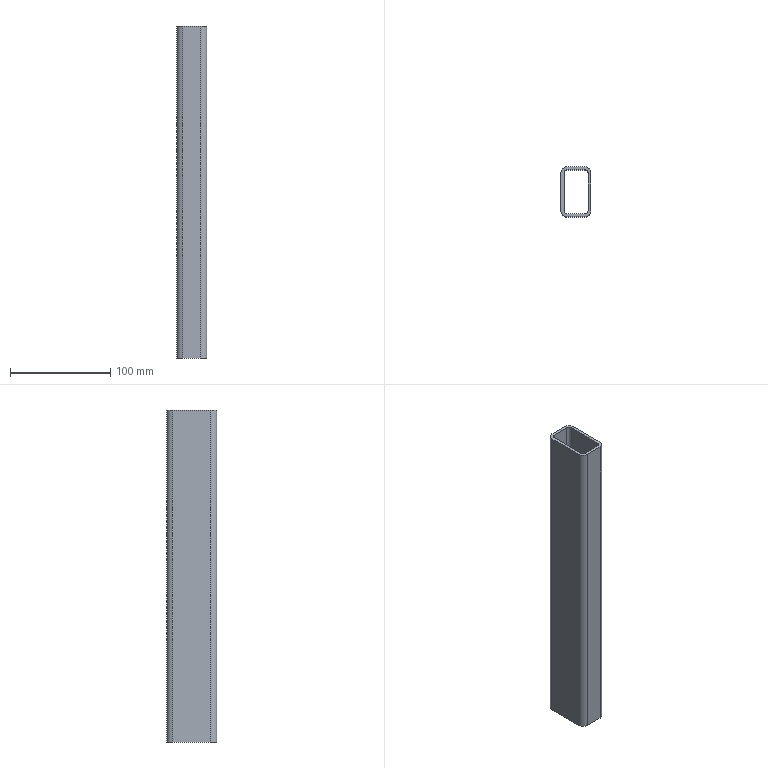Part | STEP file | ISO 10799-2 50x30x3 1784900903573 | 1 solid | 18 faces | box 30 x 50 x 332 mm | volume 139713 mm3 | plane 10 | cylinder 8 | commonest cylinder face diameters 6 x4 12 x4
STEP:
#1=CARTESIAN_POINT('',(-9.,-22.,372.));
#2=VERTEX_POINT('',#1);
#3=CARTESIAN_POINT('',(9.,-22.,372.));
#4=VERTEX_POINT('',#3);
#5=CARTESIAN_POINT('',(4.5,-22.,372.));
#6=DIRECTION('',(1.,0.,0.));
#7=VECTOR('',#6,10.);
#8=LINE('',#5,#7);
#9=EDGE_CURVE('',#2,#4,#8,.T.);
#10=ORIENTED_EDGE('',*,*,#9,.T.);
#11=CARTESIAN_POINT('',(9.,-22.,40.));
#12=VERTEX_POINT('',#11);
#13=CARTESIAN_POINT('',(9.,-22.,0.));
#14=DIRECTION('',(0.,0.,1.));
#15=VECTOR('',#14,10.);
#16=LINE('',#13,#15);
#17=EDGE_CURVE('',#12,#4,#16,.T.);
#18=ORIENTED_EDGE('',*,*,#17,.F.);
#19=CARTESIAN_POINT('',(-9.,-22.,40.));
#20=VERTEX_POINT('',#19);
#21=CARTESIAN_POINT('',(4.5,-22.,40.));
#22=DIRECTION('',(1.,0.,0.));
#23=VECTOR('',#22,10.);
#24=LINE('',#21,#23);
#25=EDGE_CURVE('',#20,#12,#24,.T.);
#26=ORIENTED_EDGE('',*,*,#25,.F.);
#27=CARTESIAN_POINT('',(-9.,-22.,0.));
#28=DIRECTION('',(0.,0.,1.));
#29=VECTOR('',#28,10.);
#30=LINE('',#27,#29);
#31=EDGE_CURVE('',#20,#2,#30,.T.);
#32=ORIENTED_EDGE('',*,*,#31,.T.);
#33=EDGE_LOOP('',(#10,#18,#26,#32));
#34=FACE_OUTER_BOUND('',#33,.T.);
#35=CARTESIAN_POINT('',(9.,-22.,0.));
#36=DIRECTION('',(0.,-1.,0.));
#37=DIRECTION('',(0.,0.,-1.));
#38=AXIS2_PLACEMENT_3D('',#35,#36,#37);
#39=PLANE('',#38);
#40=ADVANCED_FACE('',(#34),#39,.F.);
#41=CARTESIAN_POINT('',(12.,-19.,372.));
#42=VERTEX_POINT('',#41);
#43=CARTESIAN_POINT('',(9.,-19.,372.));
#44=DIRECTION('',(0.,0.,1.));
#45=DIRECTION('',(0.,1.,0.));
#46=AXIS2_PLACEMENT_3D('',#43,#44,#45);
#47=CIRCLE('',#46,3.);
#48=EDGE_CURVE('',#4,#42,#47,.T.);
#49=ORIENTED_EDGE('',*,*,#48,.T.);
#50=CARTESIAN_POINT('',(12.,-19.,40.));
#51=VERTEX_POINT('',#50);
#52=CARTESIAN_POINT('',(12.,-19.,0.));
#53=DIRECTION('',(0.,0.,1.));
#54=VECTOR('',#53,10.);
#55=LINE('',#52,#54);
#56=EDGE_CURVE('',#51,#42,#55,.T.);
#57=ORIENTED_EDGE('',*,*,#56,.F.);
#58=CARTESIAN_POINT('',(9.,-19.,40.));
#59=DIRECTION('',(0.,0.,1.));
#60=DIRECTION('',(0.,1.,0.));
#61=AXIS2_PLACEMENT_3D('',#58,#59,#60);
#62=CIRCLE('',#61,3.);
#63=EDGE_CURVE('',#12,#51,#62,.T.);
#64=ORIENTED_EDGE('',*,*,#63,.F.);
#65=ORIENTED_EDGE('',*,*,#17,.T.);
#66=EDGE_LOOP('',(#49,#57,#64,#65));
#67=FACE_OUTER_BOUND('',#66,.T.);
#68=CARTESIAN_POINT('',(9.,-19.,0.));
#69=DIRECTION('',(0.,0.,1.));
#70=DIRECTION('',(0.,1.,0.));
#71=AXIS2_PLACEMENT_3D('',#68,#69,#70);
#72=CYLINDRICAL_SURFACE('',#71,3.);
#73=ADVANCED_FACE('',(#67),#72,.F.);
#74=CARTESIAN_POINT('',(12.,19.,372.));
#75=VERTEX_POINT('',#74);
#76=CARTESIAN_POINT('',(12.,9.5,372.));
#77=DIRECTION('',(0.,1.,0.));
#78=VECTOR('',#77,10.);
#79=LINE('',#76,#78);
#80=EDGE_CURVE('',#42,#75,#79,.T.);
#81=ORIENTED_EDGE('',*,*,#80,.T.);
#82=CARTESIAN_POINT('',(12.,19.,40.));
#83=VERTEX_POINT('',#82);
#84=CARTESIAN_POINT('',(12.,19.,0.));
#85=DIRECTION('',(0.,0.,1.));
#86=VECTOR('',#85,10.);
#87=LINE('',#84,#86);
#88=EDGE_CURVE('',#83,#75,#87,.T.);
#89=ORIENTED_EDGE('',*,*,#88,.F.);
#90=CARTESIAN_POINT('',(12.,9.5,40.));
#91=DIRECTION('',(0.,1.,0.));
#92=VECTOR('',#91,10.);
#93=LINE('',#90,#92);
#94=EDGE_CURVE('',#51,#83,#93,.T.);
#95=ORIENTED_EDGE('',*,*,#94,.F.);
#96=ORIENTED_EDGE('',*,*,#56,.T.);
#97=EDGE_LOOP('',(#81,#89,#95,#96));
#98=FACE_OUTER_BOUND('',#97,.T.);
#99=CARTESIAN_POINT('',(12.,19.,0.));
#100=DIRECTION('',(1.,0.,0.));
#101=DIRECTION('',(0.,0.,-1.));
#102=AXIS2_PLACEMENT_3D('',#99,#100,#101);
#103=PLANE('',#102);
#104=ADVANCED_FACE('',(#98),#103,.F.);
#105=CARTESIAN_POINT('',(9.,22.,372.));
#106=VERTEX_POINT('',#105);
#107=CARTESIAN_POINT('',(9.,19.,372.));
#108=DIRECTION('',(0.,0.,1.));
#109=DIRECTION('',(-1.,0.,0.));
#110=AXIS2_PLACEMENT_3D('',#107,#108,#109);
#111=CIRCLE('',#110,3.);
#112=EDGE_CURVE('',#75,#106,#111,.T.);
#113=ORIENTED_EDGE('',*,*,#112,.T.);
#114=CARTESIAN_POINT('',(9.,22.,40.));
#115=VERTEX_POINT('',#114);
#116=CARTESIAN_POINT('',(9.,22.,0.));
#117=DIRECTION('',(0.,0.,1.));
#118=VECTOR('',#117,10.);
#119=LINE('',#116,#118);
#120=EDGE_CURVE('',#115,#106,#119,.T.);
#121=ORIENTED_EDGE('',*,*,#120,.F.);
#122=CARTESIAN_POINT('',(9.,19.,40.));
#123=DIRECTION('',(0.,0.,1.));
#124=DIRECTION('',(-1.,0.,0.));
#125=AXIS2_PLACEMENT_3D('',#122,#123,#124);
#126=CIRCLE('',#125,3.);
#127=EDGE_CURVE('',#83,#115,#126,.T.);
#128=ORIENTED_EDGE('',*,*,#127,.F.);
#129=ORIENTED_EDGE('',*,*,#88,.T.);
#130=EDGE_LOOP('',(#113,#121,#128,#129));
#131=FACE_OUTER_BOUND('',#130,.T.);
#132=CARTESIAN_POINT('',(9.,19.,0.));
#133=DIRECTION('',(0.,0.,1.));
#134=DIRECTION('',(-1.,0.,0.));
#135=AXIS2_PLACEMENT_3D('',#132,#133,#134);
#136=CYLINDRICAL_SURFACE('',#135,3.);
#137=ADVANCED_FACE('',(#131),#136,.F.);
#138=CARTESIAN_POINT('',(15.,19.,372.));
#139=VERTEX_POINT('',#138);
#140=CARTESIAN_POINT('',(15.,-19.,372.));
#141=VERTEX_POINT('',#140);
#142=CARTESIAN_POINT('',(15.,9.5,372.));
#143=DIRECTION('',(0.,-1.,0.));
#144=VECTOR('',#143,10.);
#145=LINE('',#142,#144);
#146=EDGE_CURVE('',#139,#141,#145,.T.);
#147=ORIENTED_EDGE('',*,*,#146,.T.);
#148=CARTESIAN_POINT('',(15.,-19.,40.));
#149=VERTEX_POINT('',#148);
#150=CARTESIAN_POINT('',(15.,-19.,0.));
#151=DIRECTION('',(0.,0.,1.));
#152=VECTOR('',#151,10.);
#153=LINE('',#150,#152);
#154=EDGE_CURVE('',#149,#141,#153,.T.);
#155=ORIENTED_EDGE('',*,*,#154,.F.);
#156=CARTESIAN_POINT('',(15.,19.,40.));
#157=VERTEX_POINT('',#156);
#158=CARTESIAN_POINT('',(15.,9.5,40.));
#159=DIRECTION('',(0.,-1.,0.));
#160=VECTOR('',#159,10.);
#161=LINE('',#158,#160);
#162=EDGE_CURVE('',#157,#149,#161,.T.);
#163=ORIENTED_EDGE('',*,*,#162,.F.);
#164=CARTESIAN_POINT('',(15.,19.,0.));
#165=DIRECTION('',(0.,0.,1.));
#166=VECTOR('',#165,10.);
#167=LINE('',#164,#166);
#168=EDGE_CURVE('',#157,#139,#167,.T.);
#169=ORIENTED_EDGE('',*,*,#168,.T.);
#170=EDGE_LOOP('',(#147,#155,#163,#169));
#171=FACE_OUTER_BOUND('',#170,.T.);
#172=CARTESIAN_POINT('',(15.,19.,0.));
#173=DIRECTION('',(1.,0.,0.));
#174=DIRECTION('',(0.,0.,-1.));
#175=AXIS2_PLACEMENT_3D('',#172,#173,#174);
#176=PLANE('',#175);
#177=ADVANCED_FACE('',(#171),#176,.T.);
#178=CARTESIAN_POINT('',(9.,-25.,372.));
#179=VERTEX_POINT('',#178);
#180=CARTESIAN_POINT('',(9.,-19.,372.));
#181=DIRECTION('',(0.,0.,-1.));
#182=DIRECTION('',(0.,1.,0.));
#183=AXIS2_PLACEMENT_3D('',#180,#181,#182);
#184=CIRCLE('',#183,6.);
#185=EDGE_CURVE('',#141,#179,#184,.T.);
#186=ORIENTED_EDGE('',*,*,#185,.T.);
#187=CARTESIAN_POINT('',(9.,-25.,40.));
#188=VERTEX_POINT('',#187);
#189=CARTESIAN_POINT('',(9.,-25.,0.));
#190=DIRECTION('',(0.,0.,1.));
#191=VECTOR('',#190,10.);
#192=LINE('',#189,#191);
#193=EDGE_CURVE('',#188,#179,#192,.T.);
#194=ORIENTED_EDGE('',*,*,#193,.F.);
#195=CARTESIAN_POINT('',(9.,-19.,40.));
#196=DIRECTION('',(0.,0.,-1.));
#197=DIRECTION('',(0.,1.,0.));
#198=AXIS2_PLACEMENT_3D('',#195,#196,#197);
#199=CIRCLE('',#198,6.);
#200=EDGE_CURVE('',#149,#188,#199,.T.);
#201=ORIENTED_EDGE('',*,*,#200,.F.);
#202=ORIENTED_EDGE('',*,*,#154,.T.);
#203=EDGE_LOOP('',(#186,#194,#201,#202));
#204=FACE_OUTER_BOUND('',#203,.T.);
#205=CARTESIAN_POINT('',(9.,-19.,0.));
#206=DIRECTION('',(0.,0.,1.));
#207=DIRECTION('',(0.,1.,0.));
#208=AXIS2_PLACEMENT_3D('',#205,#206,#207);
#209=CYLINDRICAL_SURFACE('',#208,6.);
#210=ADVANCED_FACE('',(#204),#209,.T.);
#211=CARTESIAN_POINT('',(-9.,-25.,372.));
#212=VERTEX_POINT('',#211);
#213=CARTESIAN_POINT('',(4.5,-25.,372.));
#214=DIRECTION('',(-1.,0.,0.));
#215=VECTOR('',#214,10.);
#216=LINE('',#213,#215);
#217=EDGE_CURVE('',#179,#212,#216,.T.);
#218=ORIENTED_EDGE('',*,*,#217,.T.);
#219=CARTESIAN_POINT('',(-9.,-25.,40.));
#220=VERTEX_POINT('',#219);
#221=CARTESIAN_POINT('',(-9.,-25.,0.));
#222=DIRECTION('',(0.,0.,1.));
#223=VECTOR('',#222,10.);
#224=LINE('',#221,#223);
#225=EDGE_CURVE('',#220,#212,#224,.T.);
#226=ORIENTED_EDGE('',*,*,#225,.F.);
#227=CARTESIAN_POINT('',(4.5,-25.,40.));
#228=DIRECTION('',(-1.,0.,0.));
#229=VECTOR('',#228,10.);
#230=LINE('',#227,#229);
#231=EDGE_CURVE('',#188,#220,#230,.T.);
#232=ORIENTED_EDGE('',*,*,#231,.F.);
#233=ORIENTED_EDGE('',*,*,#193,.T.);
#234=EDGE_LOOP('',(#218,#226,#232,#233));
#235=FACE_OUTER_BOUND('',#234,.T.);
#236=CARTESIAN_POINT('',(9.,-25.,0.));
#237=DIRECTION('',(0.,-1.,0.));
#238=DIRECTION('',(0.,0.,-1.));
#239=AXIS2_PLACEMENT_3D('',#236,#237,#238);
#240=PLANE('',#239);
#241=ADVANCED_FACE('',(#235),#240,.T.);
#242=CARTESIAN_POINT('',(-15.,-19.,372.));
#243=VERTEX_POINT('',#242);
#244=CARTESIAN_POINT('',(-9.,-19.,372.));
#245=DIRECTION('',(0.,0.,-1.));
#246=DIRECTION('',(1.,0.,0.));
#247=AXIS2_PLACEMENT_3D('',#244,#245,#246);
#248=CIRCLE('',#247,6.);
#249=EDGE_CURVE('',#212,#243,#248,.T.);
#250=ORIENTED_EDGE('',*,*,#249,.T.);
#251=CARTESIAN_POINT('',(-15.,-19.,40.));
#252=VERTEX_POINT('',#251);
#253=CARTESIAN_POINT('',(-15.,-19.,0.));
#254=DIRECTION('',(0.,0.,1.));
#255=VECTOR('',#254,10.);
#256=LINE('',#253,#255);
#257=EDGE_CURVE('',#252,#243,#256,.T.);
#258=ORIENTED_EDGE('',*,*,#257,.F.);
#259=CARTESIAN_POINT('',(-9.,-19.,40.));
#260=DIRECTION('',(0.,0.,-1.));
#261=DIRECTION('',(1.,0.,0.));
#262=AXIS2_PLACEMENT_3D('',#259,#260,#261);
#263=CIRCLE('',#262,6.);
#264=EDGE_CURVE('',#220,#252,#263,.T.);
#265=ORIENTED_EDGE('',*,*,#264,.F.);
#266=ORIENTED_EDGE('',*,*,#225,.T.);
#267=EDGE_LOOP('',(#250,#258,#265,#266));
#268=FACE_OUTER_BOUND('',#267,.T.);
#269=CARTESIAN_POINT('',(-9.,-19.,0.));
#270=DIRECTION('',(0.,0.,1.));
#271=DIRECTION('',(1.,0.,0.));
#272=AXIS2_PLACEMENT_3D('',#269,#270,#271);
#273=CYLINDRICAL_SURFACE('',#272,6.);
#274=ADVANCED_FACE('',(#268),#273,.T.);
#275=CARTESIAN_POINT('',(-9.,22.,372.));
#276=VERTEX_POINT('',#275);
#277=CARTESIAN_POINT('',(-4.5,22.,372.));
#278=DIRECTION('',(-1.,0.,0.));
#279=VECTOR('',#278,10.);
#280=LINE('',#277,#279);
#281=EDGE_CURVE('',#106,#276,#280,.T.);
#282=ORIENTED_EDGE('',*,*,#281,.T.);
#283=CARTESIAN_POINT('',(-9.,22.,40.));
#284=VERTEX_POINT('',#283);
#285=CARTESIAN_POINT('',(-9.,22.,0.));
#286=DIRECTION('',(0.,0.,1.));
#287=VECTOR('',#286,10.);
#288=LINE('',#285,#287);
#289=EDGE_CURVE('',#284,#276,#288,.T.);
#290=ORIENTED_EDGE('',*,*,#289,.F.);
#291=CARTESIAN_POINT('',(-4.5,22.,40.));
#292=DIRECTION('',(-1.,0.,0.));
#293=VECTOR('',#292,10.);
#294=LINE('',#291,#293);
#295=EDGE_CURVE('',#115,#284,#294,.T.);
#296=ORIENTED_EDGE('',*,*,#295,.F.);
#297=ORIENTED_EDGE('',*,*,#120,.T.);
#298=EDGE_LOOP('',(#282,#290,#296,#297));
#299=FACE_OUTER_BOUND('',#298,.T.);
#300=CARTESIAN_POINT('',(-9.,22.,0.));
#301=DIRECTION('',(0.,1.,0.));
#302=DIRECTION('',(0.,0.,1.));
#303=AXIS2_PLACEMENT_3D('',#300,#301,#302);
#304=PLANE('',#303);
#305=ADVANCED_FACE('',(#299),#304,.F.);
#306=CARTESIAN_POINT('',(-12.,-19.,372.));
#307=VERTEX_POINT('',#306);
#308=CARTESIAN_POINT('',(-9.,-19.,372.));
#309=DIRECTION('',(0.,0.,1.));
#310=DIRECTION('',(1.,0.,0.));
#311=AXIS2_PLACEMENT_3D('',#308,#309,#310);
#312=CIRCLE('',#311,3.);
#313=EDGE_CURVE('',#307,#2,#312,.T.);
#314=ORIENTED_EDGE('',*,*,#313,.T.);
#315=ORIENTED_EDGE('',*,*,#31,.F.);
#316=CARTESIAN_POINT('',(-12.,-19.,40.));
#317=VERTEX_POINT('',#316);
#318=CARTESIAN_POINT('',(-9.,-19.,40.));
#319=DIRECTION('',(0.,0.,1.));
#320=DIRECTION('',(1.,0.,0.));
#321=AXIS2_PLACEMENT_3D('',#318,#319,#320);
#322=CIRCLE('',#321,3.);
#323=EDGE_CURVE('',#317,#20,#322,.T.);
#324=ORIENTED_EDGE('',*,*,#323,.F.);
#325=CARTESIAN_POINT('',(-12.,-19.,0.));
#326=DIRECTION('',(0.,0.,1.));
#327=VECTOR('',#326,10.);
#328=LINE('',#325,#327);
#329=EDGE_CURVE('',#317,#307,#328,.T.);
#330=ORIENTED_EDGE('',*,*,#329,.T.);
#331=EDGE_LOOP('',(#314,#315,#324,#330));
#332=FACE_OUTER_BOUND('',#331,.T.);
#333=CARTESIAN_POINT('',(-9.,-19.,0.));
#334=DIRECTION('',(0.,0.,1.));
#335=DIRECTION('',(1.,0.,0.));
#336=AXIS2_PLACEMENT_3D('',#333,#334,#335);
#337=CYLINDRICAL_SURFACE('',#336,3.);
#338=ADVANCED_FACE('',(#332),#337,.F.);
#339=CARTESIAN_POINT('',(-12.,19.,372.));
#340=VERTEX_POINT('',#339);
#341=CARTESIAN_POINT('',(-12.,-9.5,372.));
#342=DIRECTION('',(0.,-1.,0.));
#343=VECTOR('',#342,10.);
#344=LINE('',#341,#343);
#345=EDGE_CURVE('',#340,#307,#344,.T.);
#346=ORIENTED_EDGE('',*,*,#345,.T.);
#347=ORIENTED_EDGE('',*,*,#329,.F.);
#348=CARTESIAN_POINT('',(-12.,19.,40.));
#349=VERTEX_POINT('',#348);
#350=CARTESIAN_POINT('',(-12.,-9.5,40.));
#351=DIRECTION('',(0.,-1.,0.));
#352=VECTOR('',#351,10.);
#353=LINE('',#350,#352);
#354=EDGE_CURVE('',#349,#317,#353,.T.);
#355=ORIENTED_EDGE('',*,*,#354,.F.);
#356=CARTESIAN_POINT('',(-12.,19.,0.));
#357=DIRECTION('',(0.,0.,1.));
#358=VECTOR('',#357,10.);
#359=LINE('',#356,#358);
#360=EDGE_CURVE('',#349,#340,#359,.T.);
#361=ORIENTED_EDGE('',*,*,#360,.T.);
#362=EDGE_LOOP('',(#346,#347,#355,#361));
#363=FACE_OUTER_BOUND('',#362,.T.);
#364=CARTESIAN_POINT('',(-12.,-19.,0.));
#365=DIRECTION('',(-1.,0.,0.));
#366=DIRECTION('',(0.,0.,1.));
#367=AXIS2_PLACEMENT_3D('',#364,#365,#366);
#368=PLANE('',#367);
#369=ADVANCED_FACE('',(#363),#368,.F.);
#370=CARTESIAN_POINT('',(-9.,19.,372.));
#371=DIRECTION('',(0.,0.,1.));
#372=DIRECTION('',(0.,-1.,0.));
#373=AXIS2_PLACEMENT_3D('',#370,#371,#372);
#374=CIRCLE('',#373,3.);
#375=EDGE_CURVE('',#276,#340,#374,.T.);
#376=ORIENTED_EDGE('',*,*,#375,.T.);
#377=ORIENTED_EDGE('',*,*,#360,.F.);
#378=CARTESIAN_POINT('',(-9.,19.,40.));
#379=DIRECTION('',(0.,0.,1.));
#380=DIRECTION('',(0.,-1.,0.));
#381=AXIS2_PLACEMENT_3D('',#378,#379,#380);
#382=CIRCLE('',#381,3.);
#383=EDGE_CURVE('',#284,#349,#382,.T.);
#384=ORIENTED_EDGE('',*,*,#383,.F.);
#385=ORIENTED_EDGE('',*,*,#289,.T.);
#386=EDGE_LOOP('',(#376,#377,#384,#385));
#387=FACE_OUTER_BOUND('',#386,.T.);
#388=CARTESIAN_POINT('',(-9.,19.,0.));
#389=DIRECTION('',(0.,0.,1.));
#390=DIRECTION('',(0.,-1.,0.));
#391=AXIS2_PLACEMENT_3D('',#388,#389,#390);
#392=CYLINDRICAL_SURFACE('',#391,3.);
#393=ADVANCED_FACE('',(#387),#392,.F.);
#394=CARTESIAN_POINT('',(-15.,19.,372.));
#395=VERTEX_POINT('',#394);
#396=CARTESIAN_POINT('',(-15.,-9.5,372.));
#397=DIRECTION('',(0.,1.,0.));
#398=VECTOR('',#397,10.);
#399=LINE('',#396,#398);
#400=EDGE_CURVE('',#243,#395,#399,.T.);
#401=ORIENTED_EDGE('',*,*,#400,.T.);
#402=CARTESIAN_POINT('',(-15.,19.,40.));
#403=VERTEX_POINT('',#402);
#404=CARTESIAN_POINT('',(-15.,19.,0.));
#405=DIRECTION('',(0.,0.,1.));
#406=VECTOR('',#405,10.);
#407=LINE('',#404,#406);
#408=EDGE_CURVE('',#403,#395,#407,.T.);
#409=ORIENTED_EDGE('',*,*,#408,.F.);
#410=CARTESIAN_POINT('',(-15.,-9.5,40.));
#411=DIRECTION('',(0.,1.,0.));
#412=VECTOR('',#411,10.);
#413=LINE('',#410,#412);
#414=EDGE_CURVE('',#252,#403,#413,.T.);
#415=ORIENTED_EDGE('',*,*,#414,.F.);
#416=ORIENTED_EDGE('',*,*,#257,.T.);
#417=EDGE_LOOP('',(#401,#409,#415,#416));
#418=FACE_OUTER_BOUND('',#417,.T.);
#419=CARTESIAN_POINT('',(-15.,-19.,0.));
#420=DIRECTION('',(-1.,0.,0.));
#421=DIRECTION('',(0.,0.,1.));
#422=AXIS2_PLACEMENT_3D('',#419,#420,#421);
#423=PLANE('',#422);
#424=ADVANCED_FACE('',(#418),#423,.T.);
#425=CARTESIAN_POINT('',(-9.,25.,372.));
#426=VERTEX_POINT('',#425);
#427=CARTESIAN_POINT('',(-9.,19.,372.));
#428=DIRECTION('',(0.,0.,-1.));
#429=DIRECTION('',(0.,-1.,0.));
#430=AXIS2_PLACEMENT_3D('',#427,#428,#429);
#431=CIRCLE('',#430,6.);
#432=EDGE_CURVE('',#395,#426,#431,.T.);
#433=ORIENTED_EDGE('',*,*,#432,.T.);
#434=CARTESIAN_POINT('',(-9.,25.,40.));
#435=VERTEX_POINT('',#434);
#436=CARTESIAN_POINT('',(-9.,25.,0.));
#437=DIRECTION('',(0.,0.,1.));
#438=VECTOR('',#437,10.);
#439=LINE('',#436,#438);
#440=EDGE_CURVE('',#435,#426,#439,.T.);
#441=ORIENTED_EDGE('',*,*,#440,.F.);
#442=CARTESIAN_POINT('',(-9.,19.,40.));
#443=DIRECTION('',(0.,0.,-1.));
#444=DIRECTION('',(0.,-1.,0.));
#445=AXIS2_PLACEMENT_3D('',#442,#443,#444);
#446=CIRCLE('',#445,6.);
#447=EDGE_CURVE('',#403,#435,#446,.T.);
#448=ORIENTED_EDGE('',*,*,#447,.F.);
#449=ORIENTED_EDGE('',*,*,#408,.T.);
#450=EDGE_LOOP('',(#433,#441,#448,#449));
#451=FACE_OUTER_BOUND('',#450,.T.);
#452=CARTESIAN_POINT('',(-9.,19.,0.));
#453=DIRECTION('',(0.,0.,1.));
#454=DIRECTION('',(0.,-1.,0.));
#455=AXIS2_PLACEMENT_3D('',#452,#453,#454);
#456=CYLINDRICAL_SURFACE('',#455,6.);
#457=ADVANCED_FACE('',(#451),#456,.T.);
#458=CARTESIAN_POINT('',(9.,25.,372.));
#459=VERTEX_POINT('',#458);
#460=CARTESIAN_POINT('',(-4.5,25.,372.));
#461=DIRECTION('',(1.,0.,0.));
#462=VECTOR('',#461,10.);
#463=LINE('',#460,#462);
#464=EDGE_CURVE('',#426,#459,#463,.T.);
#465=ORIENTED_EDGE('',*,*,#464,.T.);
#466=CARTESIAN_POINT('',(9.,25.,40.));
#467=VERTEX_POINT('',#466);
#468=CARTESIAN_POINT('',(9.,25.,0.));
#469=DIRECTION('',(0.,0.,1.));
#470=VECTOR('',#469,10.);
#471=LINE('',#468,#470);
#472=EDGE_CURVE('',#467,#459,#471,.T.);
#473=ORIENTED_EDGE('',*,*,#472,.F.);
#474=CARTESIAN_POINT('',(-4.5,25.,40.));
#475=DIRECTION('',(1.,0.,0.));
#476=VECTOR('',#475,10.);
#477=LINE('',#474,#476);
#478=EDGE_CURVE('',#435,#467,#477,.T.);
#479=ORIENTED_EDGE('',*,*,#478,.F.);
#480=ORIENTED_EDGE('',*,*,#440,.T.);
#481=EDGE_LOOP('',(#465,#473,#479,#480));
#482=FACE_OUTER_BOUND('',#481,.T.);
#483=CARTESIAN_POINT('',(-9.,25.,0.));
#484=DIRECTION('',(0.,1.,0.));
#485=DIRECTION('',(0.,0.,1.));
#486=AXIS2_PLACEMENT_3D('',#483,#484,#485);
#487=PLANE('',#486);
#488=ADVANCED_FACE('',(#482),#487,.T.);
#489=CARTESIAN_POINT('',(9.,19.,372.));
#490=DIRECTION('',(0.,0.,-1.));
#491=DIRECTION('',(-1.,0.,0.));
#492=AXIS2_PLACEMENT_3D('',#489,#490,#491);
#493=CIRCLE('',#492,6.);
#494=EDGE_CURVE('',#459,#139,#493,.T.);
#495=ORIENTED_EDGE('',*,*,#494,.T.);
#496=ORIENTED_EDGE('',*,*,#168,.F.);
#497=CARTESIAN_POINT('',(9.,19.,40.));
#498=DIRECTION('',(0.,0.,-1.));
#499=DIRECTION('',(-1.,0.,0.));
#500=AXIS2_PLACEMENT_3D('',#497,#498,#499);
#501=CIRCLE('',#500,6.);
#502=EDGE_CURVE('',#467,#157,#501,.T.);
#503=ORIENTED_EDGE('',*,*,#502,.F.);
#504=ORIENTED_EDGE('',*,*,#472,.T.);
#505=EDGE_LOOP('',(#495,#496,#503,#504));
#506=FACE_OUTER_BOUND('',#505,.T.);
#507=CARTESIAN_POINT('',(9.,19.,0.));
#508=DIRECTION('',(0.,0.,1.));
#509=DIRECTION('',(-1.,0.,0.));
#510=AXIS2_PLACEMENT_3D('',#507,#508,#509);
#511=CYLINDRICAL_SURFACE('',#510,6.);
#512=ADVANCED_FACE('',(#506),#511,.T.);
#513=ORIENTED_EDGE('',*,*,#414,.T.);
#514=ORIENTED_EDGE('',*,*,#447,.T.);
#515=ORIENTED_EDGE('',*,*,#478,.T.);
#516=ORIENTED_EDGE('',*,*,#502,.T.);
#517=ORIENTED_EDGE('',*,*,#162,.T.);
#518=ORIENTED_EDGE('',*,*,#200,.T.);
#519=ORIENTED_EDGE('',*,*,#231,.T.);
#520=ORIENTED_EDGE('',*,*,#264,.T.);
#521=EDGE_LOOP('',(#513,#514,#515,#516,#517,#518,#519,#520));
#522=FACE_OUTER_BOUND('',#521,.T.);
#523=ORIENTED_EDGE('',*,*,#295,.T.);
#524=ORIENTED_EDGE('',*,*,#383,.T.);
#525=ORIENTED_EDGE('',*,*,#354,.T.);
#526=ORIENTED_EDGE('',*,*,#323,.T.);
#527=ORIENTED_EDGE('',*,*,#25,.T.);
#528=ORIENTED_EDGE('',*,*,#63,.T.);
#529=ORIENTED_EDGE('',*,*,#94,.T.);
#530=ORIENTED_EDGE('',*,*,#127,.T.);
#531=EDGE_LOOP('',(#523,#524,#525,#526,#527,#528,#529,#530));
#532=FACE_BOUND('',#531,.T.);
#533=CARTESIAN_POINT('',(0.,0.,40.));
#534=DIRECTION('',(0.,0.,1.));
#535=DIRECTION('',(1.,0.,0.));
#536=AXIS2_PLACEMENT_3D('',#533,#534,#535);
#537=PLANE('',#536);
#538=ADVANCED_FACE('',(#522,#532),#537,.F.);
#539=ORIENTED_EDGE('',*,*,#400,.F.);
#540=ORIENTED_EDGE('',*,*,#249,.F.);
#541=ORIENTED_EDGE('',*,*,#217,.F.);
#542=ORIENTED_EDGE('',*,*,#185,.F.);
#543=ORIENTED_EDGE('',*,*,#146,.F.);
#544=ORIENTED_EDGE('',*,*,#494,.F.);
#545=ORIENTED_EDGE('',*,*,#464,.F.);
#546=ORIENTED_EDGE('',*,*,#432,.F.);
#547=EDGE_LOOP('',(#539,#540,#541,#542,#543,#544,#545,#546));
#548=FACE_OUTER_BOUND('',#547,.T.);
#549=ORIENTED_EDGE('',*,*,#281,.F.);
#550=ORIENTED_EDGE('',*,*,#112,.F.);
#551=ORIENTED_EDGE('',*,*,#80,.F.);
#552=ORIENTED_EDGE('',*,*,#48,.F.);
#553=ORIENTED_EDGE('',*,*,#9,.F.);
#554=ORIENTED_EDGE('',*,*,#313,.F.);
#555=ORIENTED_EDGE('',*,*,#345,.F.);
#556=ORIENTED_EDGE('',*,*,#375,.F.);
#557=EDGE_LOOP('',(#549,#550,#551,#552,#553,#554,#555,#556));
#558=FACE_BOUND('',#557,.T.);
#559=CARTESIAN_POINT('',(0.,0.,372.));
#560=DIRECTION('',(0.,0.,1.));
#561=DIRECTION('',(1.,0.,0.));
#562=AXIS2_PLACEMENT_3D('',#559,#560,#561);
#563=PLANE('',#562);
#564=ADVANCED_FACE('',(#548,#558),#563,.T.);
#565=CLOSED_SHELL('',(#40,#73,#104,#137,#177,#210,#241,#274,#305,#338,#369,#393,#424,#457,#488,#512,#538,#564));
#566=MANIFOLD_SOLID_BREP('',#565);
#567=(LENGTH_UNIT()NAMED_UNIT(*)SI_UNIT(.MILLI.,.METRE.));
#568=UNCERTAINTY_MEASURE_WITH_UNIT(LENGTH_MEASURE(0.01),#567,'','');
#569=(NAMED_UNIT(*)PLANE_ANGLE_UNIT()SI_UNIT($,.RADIAN.));
#570=(NAMED_UNIT(*)SI_UNIT($,.STERADIAN.)SOLID_ANGLE_UNIT());
#571=(GEOMETRIC_REPRESENTATION_CONTEXT(3)GLOBAL_UNCERTAINTY_ASSIGNED_CONTEXT((#568))GLOBAL_UNIT_ASSIGNED_CONTEXT((#567,#569,#570))REPRESENTATION_CONTEXT('',''));
#572=ADVANCED_BREP_SHAPE_REPRESENTATION('',(#566),#571);